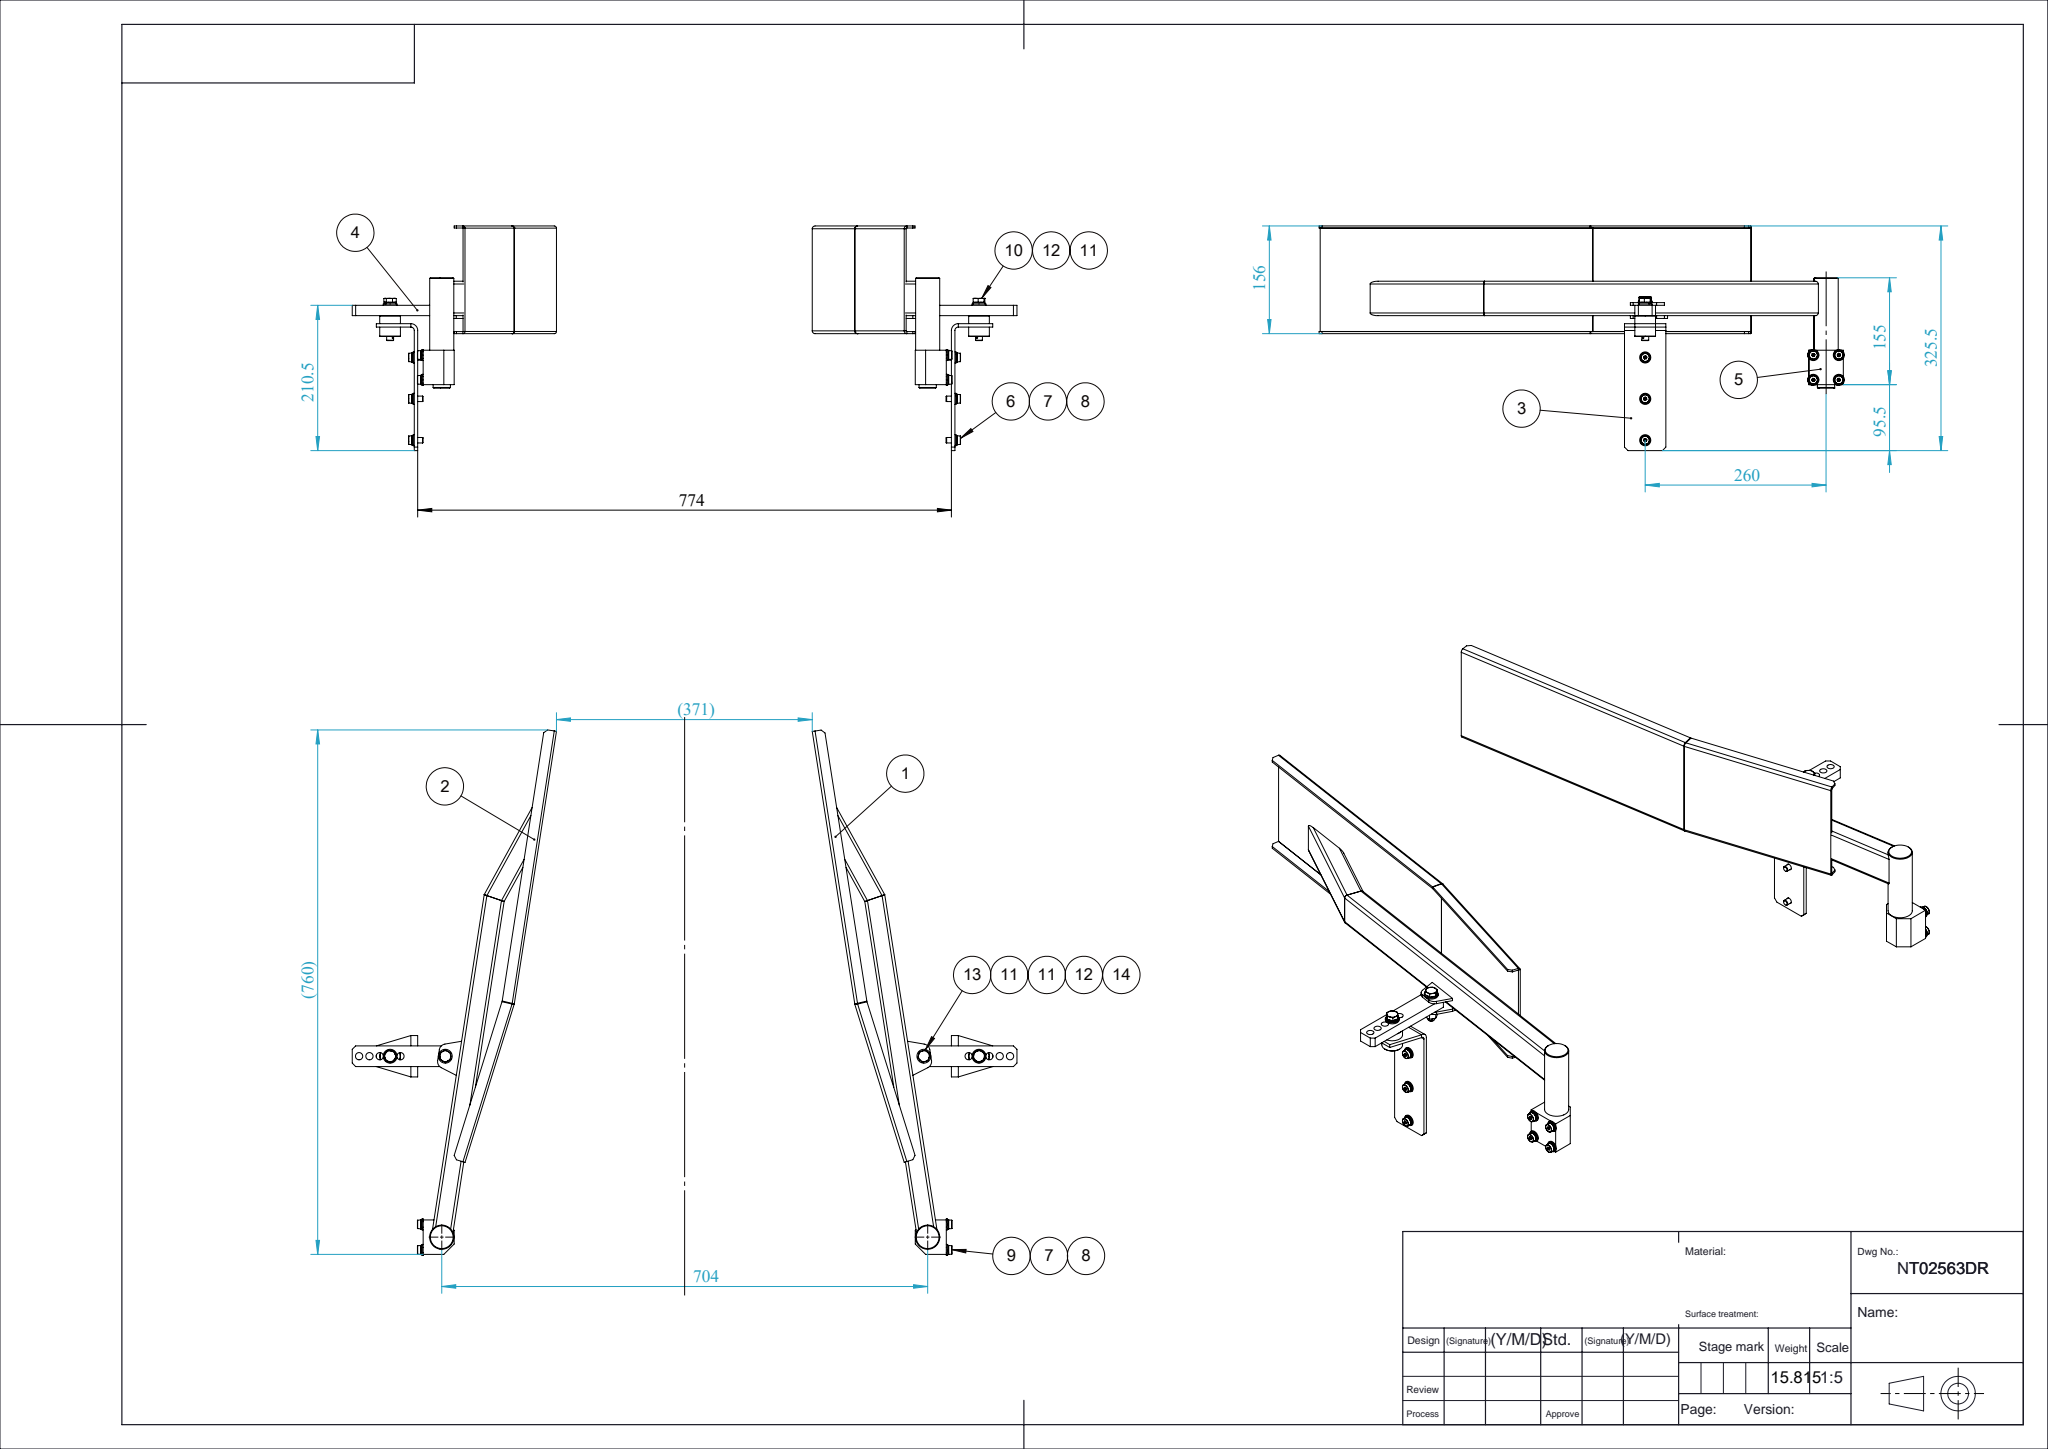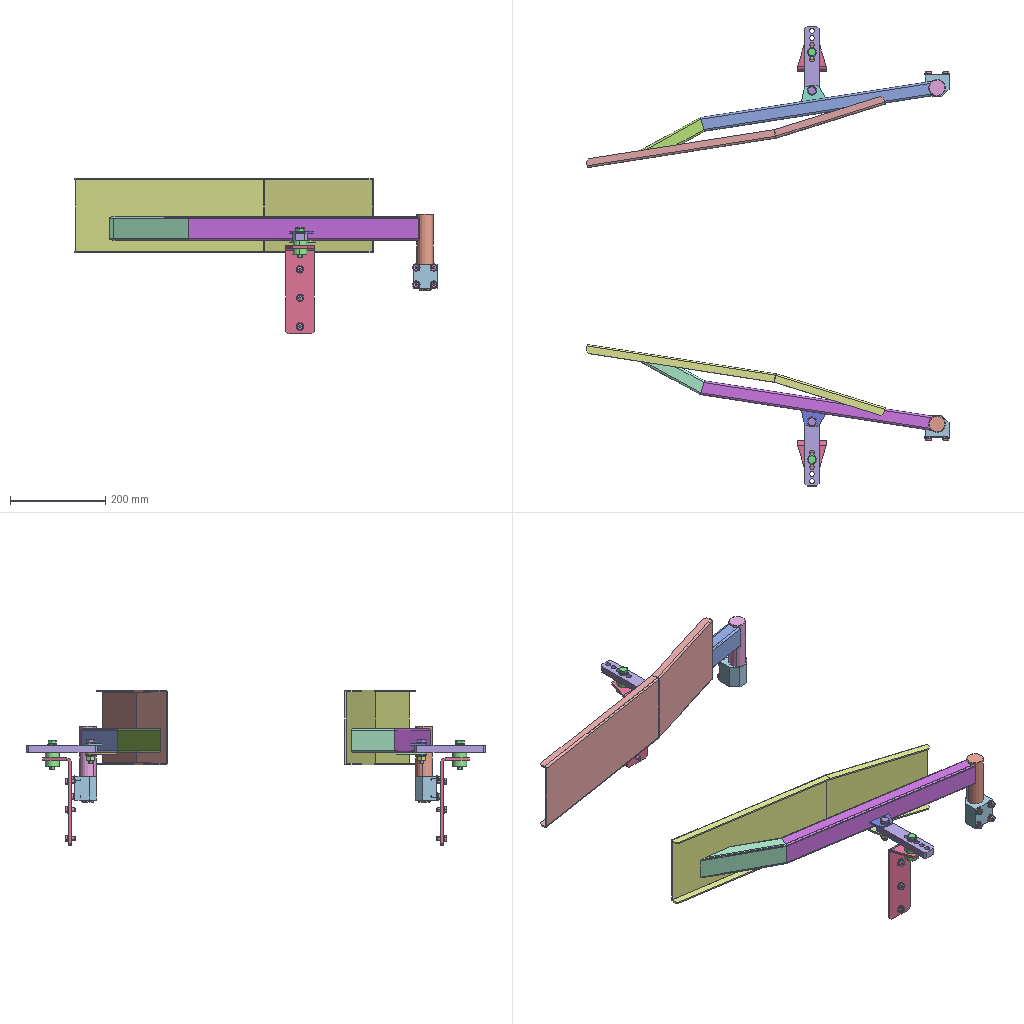Assembly | SolidWorks | 24 different items | 29 placed | box 762 x 964 x 326 mm
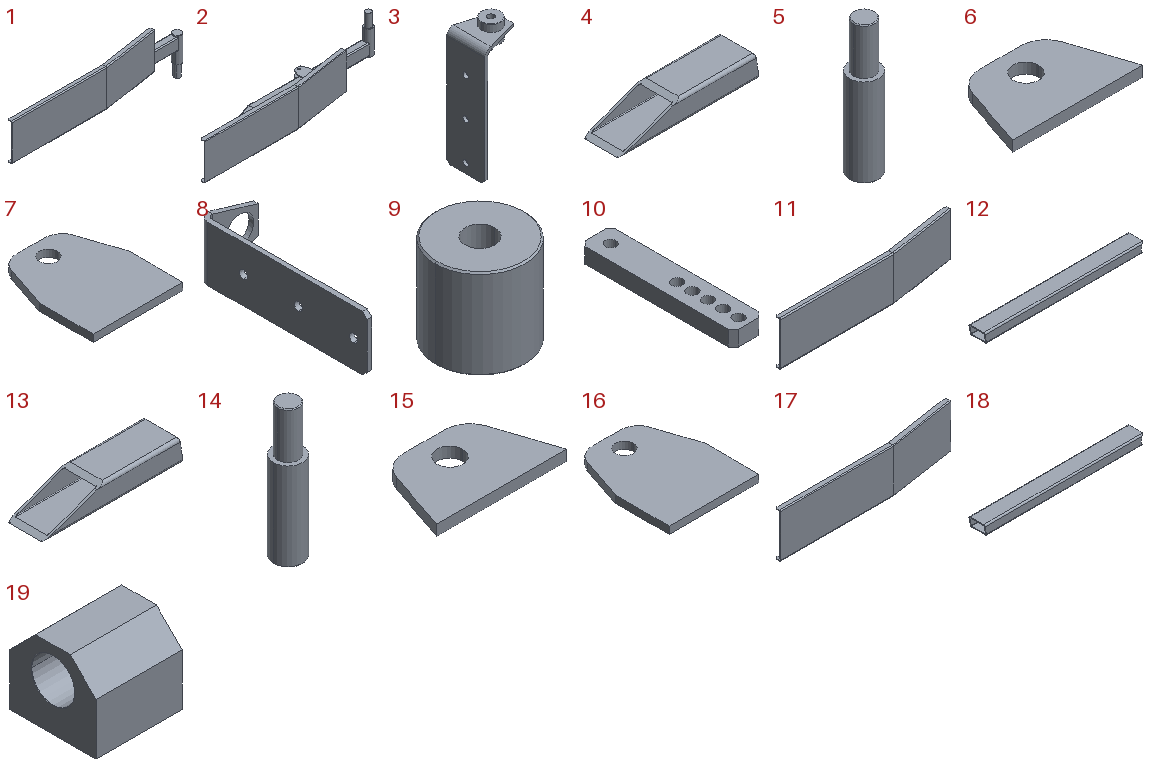Parts list (item | name | quantity | parent item | size | volume | features):
1 | (subassembly) | x1 | - | 767.5 x 97.3 x 235 mm | 766450 mm3 | features CompositeCurve 7
2 | (subassembly) | x1 | - | 767.5 x 97.3 x 235 mm | 768055 mm3 | features CompositeCurve 2
3 | (subassembly) | x2 | - | 60 x 60 x 195.5 mm | 81197 mm3 | -
4 | - | x1 | in 2 | 188 x 50 x 30 mm | 62143 mm3 | features ICE 2, WeldMemberFeat 1, WeldmentFeature 1
5 | - | x1 | in 2 | 35 x 35 x 160 mm | 127928 mm3 | features Chamfer 1, Extrusion 1, ICE 1
6 | - | x1 | in 2 | 50 x 30 x 4 mm | 4409 mm3 | features Extrusion 1
7 | - | x1 | in 2 | 50 x 60 x 4 mm | 10409 mm3 | features Extrusion 1
8 | - | x2 | in 3 | 60 x 184 x 60 mm | 62371 mm3 | features ICE 3, Chamfer 1, Extrusion 1
9 | - | x2 | in 3 | 30 x 30 x 30 mm | 18826 mm3 | features Chamfer 1, Extrusion 1
10 | - | x2 | - | 30 x 150 x 15 mm | 58957 mm3 | features Chamfer 1, Extrusion 1, ICE 1
11 | - | x1 | in 1 | 637.587 x 52.537 x 156 mm | 352629 mm3 | features EdgeFlange 2, Chamfer 1, FlatPattern 1, SMBaseFlange 1, SheetMetal 1
12 | - | x1 | in 1 | 490.986 x 50 x 30 mm | 208931 mm3 | features ICE 2, WeldMemberFeat 1, WeldmentFeature 1
13 | - | x1 | in 1 | 188 x 50 x 30 mm | 62143 mm3 | features ICE 2, WeldMemberFeat 1, WeldmentFeature 1
14 | - | x1 | in 1 | 35 x 35 x 160 mm | 127928 mm3 | features Chamfer 1, Extrusion 1, ICE 1
15 | - | x1 | in 1 | 50 x 30 x 4 mm | 4409 mm3 | features Extrusion 1
16 | - | x1 | in 1 | 50 x 60 x 4 mm | 10409 mm3 | features Extrusion 1
17 | - | x1 | in 2 | 637.807 x 52.57 x 156 mm | 354234 mm3 | features Chamfer 1, EdgeFlange 1, FlatPattern 1, SMBaseFlange 1, SheetMetal 1
18 | - | x1 | in 2 | 490.986 x 50 x 30 mm | 208931 mm3 | features ICE 2, WeldMemberFeat 1, WeldmentFeature 1
19 | - | x2 | - | 50 x 50 x 45 mm | 73670 mm3 | features Chamfer 3, Extrusion 1, HoleWzd 1, ICE 1
20 | curved single coil spring lock washers gb | x1 | - | - | - | -
21 | hex bolts split pin hole-fine pitch-ab gb | x1 | - | - | - | -
22 | hex lobular socket thread forming screws gb | x1 | - | - | - | -
23 | hex nut-fine pitch-style washer-grade ab gb | x1 | - | - | - | -
24 | plain washers--product grade c gb | x1 | - | - | - | -
Mates (type | each side: item.copy, entity, surface, feature):
In the top assembly
Coincident | 15.1 face plane Boss-Extrude1 | 10.1 face plane Boss-Extrude1
Concentric | 15.1 face cylinder Boss-Extrude1 | 10.1 face cylinder Cut-Extrude1
Coincident | 10.1 face plane Boss-Extrude1 | 9.1 face plane Boss-Extrude1
Concentric | 10.1 face cylinder Cut-Extrude1 | 9.1 face cylinder Boss-Extrude1
Parallel | 10.1 face plane Boss-Extrude1 | 8.1 face plane Boss-Extrude1
Concentric | 14.1 face cylinder Boss-Extrude2 | 19.1 face cylinder Cut-Extrude1
Coincident | 14.1 face plane Boss-Extrude1 | 19.1 face plane Boss-Extrude1
Concentric | 5.1 face cylinder Boss-Extrude2 | 19.2 face cylinder Cut-Extrude1
Coincident | 5.1 face plane Boss-Extrude1 | 19.2 face plane Boss-Extrude1
Coincident | 6.1 face plane Boss-Extrude1 | 10.2 face plane Boss-Extrude1
Concentric | 6.1 edge | 10.2 edge
Concentric | 10.2 edge | 9.2 edge
Coincident | 10.2 face plane Boss-Extrude1 | 9.2 face plane Boss-Extrude1
Coincident | 11.1 face plane Edge-Flange2 | 17.1 face plane Edge-Flange3
Parallel | 8.1 face plane Boss-Extrude1 | 8.2 face plane Boss-Extrude1
DistanceDim | 8.2 face plane Boss-Extrude1 | 8.1 face plane Boss-Extrude1
Coincident | 8.2 face plane Boss-Extrude1 | assembly plane
Parallel | 10.2 face plane Boss-Extrude1 | 8.2 face plane Boss-Extrude1
Coincident | 10.1 face plane Boss-Extrude1 | 10.2 face plane Boss-Extrude1
Parallel | 19.2 face plane Boss-Extrude1 | 8.2 face plane Boss-Extrude1
Parallel | 8.1 face plane Boss-Extrude1 | 19.1 face plane Boss-Extrude1
DistanceDim | 17.1 edge | 11.1 edge
Perpendicular | 18.1 face plane Square tube 30 X 30 X 2.6(15) | assembly plane
In subassembly 1
Concentric | 12.1 face cylinder Cut-Extrude4 | 14.2 face cylinder Boss-Extrude1
DistanceDim | 12.1 face plane Square tube 30 X 30 X 2.6(15) | 14.2 face plane Boss-Extrude2
Coincident | 12.1 face plane Cut-Extrude3 | 13.1 face plane Cut-Extrude1
Coincident | 12.1 edge | 13.1 edge | 2 times
Coincident | 12.1 face plane Square tube 30 X 30 X 2.6(15) | 16.1 face plane Boss-Extrude1
Coincident | 12.1 face plane Square tube 30 X 30 X 2.6(15) | 15.2 face plane Boss-Extrude1
Concentric | 15.2 edge | 16.1 edge
DistanceDim | 13.1 edge | 15.2 edge
DistanceDim | 15.2 face plane Boss-Extrude1 | 16.1 face plane Boss-Extrude1
Coincident | 11.2 face plane Base-Flange4 | 13.1 face plane Cut-Extrude2 | 2 times
DistanceDim | 12.1 face plane Square tube 30 X 30 X 2.6(15) | 11.2 face plane Edge-Flange2
DistanceDim | 16.1 face plane Boss-Extrude1 | 11.2 face plane Edge-Flange2
In subassembly 3
Concentric | 9.3 face cylinder Boss-Extrude1 | 8.3 face cylinder Cut-Extrude1
DistanceDim | 9.3 face plane Boss-Extrude1 | 8.3 face plane Boss-Extrude1
In subassembly 2
Coincident | 18.2 face plane Cut-Extrude3 | 4.1 face plane Cut-Extrude1
Coincident | 18.2 edge | 4.1 edge
Coincident | 18.2 edge | 4.1 face plane Square tube 30 X 30 X 2.6(1)
Concentric | 18.2 face cylinder Cut-Extrude4 | 5.2 face cylinder Boss-Extrude1
DistanceDim | 18.2 face plane Square tube 30 X 30 X 2.6(15) | 5.2 face plane Boss-Extrude2
Coincident | 18.2 face plane Square tube 30 X 30 X 2.6(15) | 6.2 face plane Boss-Extrude1
Coincident | 18.2 face plane Square tube 30 X 30 X 2.6(15) | 7.1 face plane Boss-Extrude1
Concentric | 6.2 edge | 7.1 edge
DistanceDim | 7.1 edge | 4.1 edge
Coincident | 17.2 face plane Base-Flange4 | 4.1 face plane Cut-Extrude2
DistanceDim | 18.2 face plane Square tube 30 X 30 X 2.6(15) | 17.2 face plane Edge-Flange3
DistanceDim | 6.2 face plane Boss-Extrude1 | 7.1 face plane Boss-Extrude1
DistanceDim | 7.1 face plane Boss-Extrude1 | 17.2 face plane Edge-Flange3